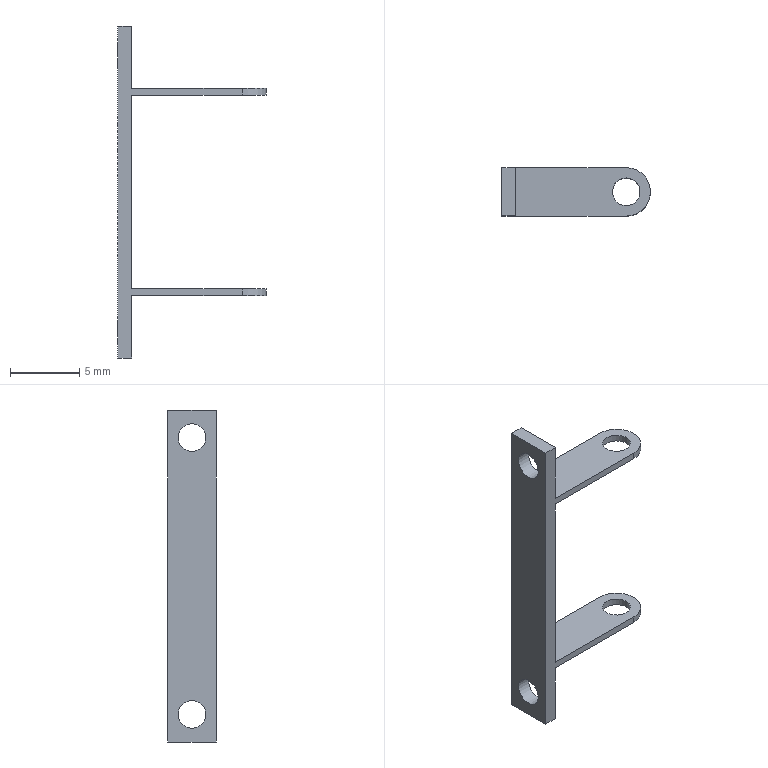Part | STEP file | 1-63.3 | 1 solid | 18 faces | box 10.75 x 3.5 x 24 mm | volume 107.386 mm3 | plane 12 | cylinder 6 | commonest cylinder face diameters 2 x4 3.5 x2
STEP:
#1=CARTESIAN_POINT('',(0.,0.,0.));
#2=DIRECTION('',(0.,0.,1.));
#3=DIRECTION('',(1.,0.,0.));
#4=AXIS2_PLACEMENT_3D('',#1,#2,#3);
#5=CARTESIAN_POINT('',(0.,-1.75,-12.));
#6=VERTEX_POINT('',#5);
#7=CARTESIAN_POINT('',(0.,1.75,-12.));
#8=VERTEX_POINT('',#7);
#9=CARTESIAN_POINT('',(0.,-1.75,-12.));
#10=DIRECTION('',(0.,1.,0.));
#11=VECTOR('',#10,1.);
#12=LINE('',#9,#11);
#13=CARTESIAN_POINT('',(0.,10.25,0.));
#14=DIRECTION('',(1.,0.,0.));
#15=DIRECTION('',(0.,1.,0.));
#16=AXIS2_PLACEMENT_3D('',#13,#14,#15);
#17=PLANE('',#16);
#18=CARTESIAN_POINT('',(-12.,-12.));
#19=DIRECTION('',(1.,0.));
#20=VECTOR('',#19,1.);
#21=LINE('',#18,#20);
#22=(GEOMETRIC_REPRESENTATION_CONTEXT(2)PARAMETRIC_REPRESENTATION_CONTEXT()REPRESENTATION_CONTEXT('',''));
#23=DEFINITIONAL_REPRESENTATION('',(#21),#22);
#24=PCURVE('',#17,#23);
#25=CARTESIAN_POINT('',(0.5,0.,-12.));
#26=DIRECTION('',(0.,0.,-1.));
#27=DIRECTION('',(0.,1.,0.));
#28=AXIS2_PLACEMENT_3D('',#25,#26,#27);
#29=PLANE('',#28);
#30=CARTESIAN_POINT('',(-1.75,-0.5));
#31=DIRECTION('',(1.,0.));
#32=VECTOR('',#31,1.);
#33=LINE('',#30,#32);
#34=(GEOMETRIC_REPRESENTATION_CONTEXT(2)PARAMETRIC_REPRESENTATION_CONTEXT()REPRESENTATION_CONTEXT('',''));
#35=DEFINITIONAL_REPRESENTATION('',(#33),#34);
#36=PCURVE('',#29,#35);
#37=SURFACE_CURVE('',#12,(#24,#36),.PCURVE_S1.);
#38=EDGE_CURVE('',#6,#8,#37,.T.);
#39=ORIENTED_EDGE('',*,*,#38,.T.);
#40=CARTESIAN_POINT('',(0.,1.75,12.));
#41=VERTEX_POINT('',#40);
#42=CARTESIAN_POINT('',(0.,1.75,-12.));
#43=DIRECTION('',(0.,0.,1.));
#44=VECTOR('',#43,1.);
#45=LINE('',#42,#44);
#46=CARTESIAN_POINT('',(-8.5,-12.));
#47=DIRECTION('',(0.,1.));
#48=VECTOR('',#47,1.);
#49=LINE('',#46,#48);
#50=(GEOMETRIC_REPRESENTATION_CONTEXT(2)PARAMETRIC_REPRESENTATION_CONTEXT()REPRESENTATION_CONTEXT('',''));
#51=DEFINITIONAL_REPRESENTATION('',(#49),#50);
#52=PCURVE('',#17,#51);
#53=CARTESIAN_POINT('',(4.5,1.75,0.));
#54=DIRECTION('',(0.,1.,0.));
#55=DIRECTION('',(0.,0.,1.));
#56=AXIS2_PLACEMENT_3D('',#53,#54,#55);
#57=PLANE('',#56);
#58=CARTESIAN_POINT('',(-12.,-4.5));
#59=DIRECTION('',(1.,0.));
#60=VECTOR('',#59,1.);
#61=LINE('',#58,#60);
#62=(GEOMETRIC_REPRESENTATION_CONTEXT(2)PARAMETRIC_REPRESENTATION_CONTEXT()REPRESENTATION_CONTEXT('',''));
#63=DEFINITIONAL_REPRESENTATION('',(#61),#62);
#64=PCURVE('',#57,#63);
#65=SURFACE_CURVE('',#45,(#52,#64),.PCURVE_S1.);
#66=EDGE_CURVE('',#8,#41,#65,.T.);
#67=ORIENTED_EDGE('',*,*,#66,.T.);
#68=CARTESIAN_POINT('',(0.,-1.75,12.));
#69=VERTEX_POINT('',#68);
#70=CARTESIAN_POINT('',(0.,1.75,12.));
#71=DIRECTION('',(0.,-1.,0.));
#72=VECTOR('',#71,1.);
#73=LINE('',#70,#72);
#74=CARTESIAN_POINT('',(-8.5,12.));
#75=DIRECTION('',(-1.,0.));
#76=VECTOR('',#75,1.);
#77=LINE('',#74,#76);
#78=(GEOMETRIC_REPRESENTATION_CONTEXT(2)PARAMETRIC_REPRESENTATION_CONTEXT()REPRESENTATION_CONTEXT('',''));
#79=DEFINITIONAL_REPRESENTATION('',(#77),#78);
#80=PCURVE('',#17,#79);
#81=CARTESIAN_POINT('',(0.5,0.,12.));
#82=DIRECTION('',(0.,0.,1.));
#83=DIRECTION('',(0.,-1.,0.));
#84=AXIS2_PLACEMENT_3D('',#81,#82,#83);
#85=PLANE('',#84);
#86=CARTESIAN_POINT('',(-1.75,-0.5));
#87=DIRECTION('',(1.,0.));
#88=VECTOR('',#87,1.);
#89=LINE('',#86,#88);
#90=(GEOMETRIC_REPRESENTATION_CONTEXT(2)PARAMETRIC_REPRESENTATION_CONTEXT()REPRESENTATION_CONTEXT('',''));
#91=DEFINITIONAL_REPRESENTATION('',(#89),#90);
#92=PCURVE('',#85,#91);
#93=SURFACE_CURVE('',#73,(#80,#92),.PCURVE_S1.);
#94=EDGE_CURVE('',#41,#69,#93,.T.);
#95=ORIENTED_EDGE('',*,*,#94,.T.);
#96=CARTESIAN_POINT('',(0.,-1.75,12.));
#97=DIRECTION('',(0.,0.,-1.));
#98=VECTOR('',#97,1.);
#99=LINE('',#96,#98);
#100=CARTESIAN_POINT('',(-12.,12.));
#101=DIRECTION('',(0.,-1.));
#102=VECTOR('',#101,1.);
#103=LINE('',#100,#102);
#104=(GEOMETRIC_REPRESENTATION_CONTEXT(2)PARAMETRIC_REPRESENTATION_CONTEXT()REPRESENTATION_CONTEXT('',''));
#105=DEFINITIONAL_REPRESENTATION('',(#103),#104);
#106=PCURVE('',#17,#105);
#107=CARTESIAN_POINT('',(4.5,-1.75,0.));
#108=DIRECTION('',(0.,-1.,0.));
#109=DIRECTION('',(0.,0.,-1.));
#110=AXIS2_PLACEMENT_3D('',#107,#108,#109);
#111=PLANE('',#110);
#112=CARTESIAN_POINT('',(-12.,-4.5));
#113=DIRECTION('',(1.,0.));
#114=VECTOR('',#113,1.);
#115=LINE('',#112,#114);
#116=(GEOMETRIC_REPRESENTATION_CONTEXT(2)PARAMETRIC_REPRESENTATION_CONTEXT()REPRESENTATION_CONTEXT('',''));
#117=DEFINITIONAL_REPRESENTATION('',(#115),#116);
#118=PCURVE('',#111,#117);
#119=SURFACE_CURVE('',#99,(#106,#118),.PCURVE_S1.);
#120=EDGE_CURVE('',#69,#6,#119,.T.);
#121=ORIENTED_EDGE('',*,*,#120,.T.);
#122=EDGE_LOOP('',(#39,#67,#95,#121));
#123=FACE_BOUND('',#122,.F.);
#124=CARTESIAN_POINT('',(0.,1.,10.));
#125=VERTEX_POINT('',#124);
#126=CARTESIAN_POINT('',(0.,0.,10.));
#127=DIRECTION('',(-1.,0.,0.));
#128=DIRECTION('',(0.,1.,0.));
#129=AXIS2_PLACEMENT_3D('',#126,#127,#128);
#130=CIRCLE('',#129,1.);
#131=CARTESIAN_POINT('',(-9.25,10.));
#132=CARTESIAN_POINT('',(-9.25,8.268));
#133=CARTESIAN_POINT('',(-10.75,9.134));
#134=CARTESIAN_POINT('',(-12.25,10.));
#135=CARTESIAN_POINT('',(-10.75,10.866));
#136=CARTESIAN_POINT('',(-9.25,11.732));
#137=CARTESIAN_POINT('',(-9.25,10.));
#138=(BOUNDED_CURVE()B_SPLINE_CURVE(2,(#131,#132,#133,#134,#135,#136,#137),.UNSPECIFIED.,.T.,.F.)B_SPLINE_CURVE_WITH_KNOTS((1,2,2,2,2,1),(-2.094,0.,2.094,4.189,6.283,8.378),.UNSPECIFIED.)CURVE()GEOMETRIC_REPRESENTATION_ITEM()RATIONAL_B_SPLINE_CURVE((1.,0.5,1.,0.5,1.,0.5,1.))REPRESENTATION_ITEM(''));
#139=(GEOMETRIC_REPRESENTATION_CONTEXT(2)PARAMETRIC_REPRESENTATION_CONTEXT()REPRESENTATION_CONTEXT('',''));
#140=DEFINITIONAL_REPRESENTATION('',(#138),#139);
#141=PCURVE('',#17,#140);
#142=CARTESIAN_POINT('',(0.,0.,10.));
#143=DIRECTION('',(1.,0.,0.));
#144=DIRECTION('',(0.,1.,0.));
#145=AXIS2_PLACEMENT_3D('',#142,#143,#144);
#146=CYLINDRICAL_SURFACE('',#145,1.);
#147=CARTESIAN_POINT('',(6.283,0.));
#148=DIRECTION('',(-1.,0.));
#149=VECTOR('',#148,1.);
#150=LINE('',#147,#149);
#151=(GEOMETRIC_REPRESENTATION_CONTEXT(2)PARAMETRIC_REPRESENTATION_CONTEXT()REPRESENTATION_CONTEXT('',''));
#152=DEFINITIONAL_REPRESENTATION('',(#150),#151);
#153=PCURVE('',#146,#152);
#154=SURFACE_CURVE('',#130,(#141,#153),.PCURVE_S1.);
#155=EDGE_CURVE('',#125,#125,#154,.T.);
#156=ORIENTED_EDGE('',*,*,#155,.T.);
#157=EDGE_LOOP('',(#156));
#158=FACE_BOUND('',#157,.F.);
#159=CARTESIAN_POINT('',(0.,1.,-10.));
#160=VERTEX_POINT('',#159);
#161=CARTESIAN_POINT('',(0.,0.,-10.));
#162=DIRECTION('',(-1.,0.,0.));
#163=DIRECTION('',(0.,1.,0.));
#164=AXIS2_PLACEMENT_3D('',#161,#162,#163);
#165=CIRCLE('',#164,1.);
#166=CARTESIAN_POINT('',(-9.25,-10.));
#167=CARTESIAN_POINT('',(-9.25,-11.732));
#168=CARTESIAN_POINT('',(-10.75,-10.866));
#169=CARTESIAN_POINT('',(-12.25,-10.));
#170=CARTESIAN_POINT('',(-10.75,-9.134));
#171=CARTESIAN_POINT('',(-9.25,-8.268));
#172=CARTESIAN_POINT('',(-9.25,-10.));
#173=(BOUNDED_CURVE()B_SPLINE_CURVE(2,(#166,#167,#168,#169,#170,#171,#172),.UNSPECIFIED.,.T.,.F.)B_SPLINE_CURVE_WITH_KNOTS((1,2,2,2,2,1),(-2.094,0.,2.094,4.189,6.283,8.378),.UNSPECIFIED.)CURVE()GEOMETRIC_REPRESENTATION_ITEM()RATIONAL_B_SPLINE_CURVE((1.,0.5,1.,0.5,1.,0.5,1.))REPRESENTATION_ITEM(''));
#174=(GEOMETRIC_REPRESENTATION_CONTEXT(2)PARAMETRIC_REPRESENTATION_CONTEXT()REPRESENTATION_CONTEXT('',''));
#175=DEFINITIONAL_REPRESENTATION('',(#173),#174);
#176=PCURVE('',#17,#175);
#177=CARTESIAN_POINT('',(0.,0.,-10.));
#178=DIRECTION('',(1.,0.,0.));
#179=DIRECTION('',(0.,1.,0.));
#180=AXIS2_PLACEMENT_3D('',#177,#178,#179);
#181=CYLINDRICAL_SURFACE('',#180,1.);
#182=CARTESIAN_POINT('',(6.283,0.));
#183=DIRECTION('',(-1.,0.));
#184=VECTOR('',#183,1.);
#185=LINE('',#182,#184);
#186=(GEOMETRIC_REPRESENTATION_CONTEXT(2)PARAMETRIC_REPRESENTATION_CONTEXT()REPRESENTATION_CONTEXT('',''));
#187=DEFINITIONAL_REPRESENTATION('',(#185),#186);
#188=PCURVE('',#181,#187);
#189=SURFACE_CURVE('',#165,(#176,#188),.PCURVE_S1.);
#190=EDGE_CURVE('',#160,#160,#189,.T.);
#191=ORIENTED_EDGE('',*,*,#190,.T.);
#192=EDGE_LOOP('',(#191));
#193=FACE_BOUND('',#192,.F.);
#194=ADVANCED_FACE('',(#123,#158,#193),#17,.F.);
#195=ORIENTED_EDGE('',*,*,#38,.T.);
#196=CARTESIAN_POINT('',(1.,1.75,-12.));
#197=VERTEX_POINT('',#196);
#198=CARTESIAN_POINT('',(0.,1.75,-12.));
#199=DIRECTION('',(1.,0.,0.));
#200=VECTOR('',#199,1.);
#201=LINE('',#198,#200);
#202=CARTESIAN_POINT('',(1.75,-0.5));
#203=DIRECTION('',(0.,1.));
#204=VECTOR('',#203,1.);
#205=LINE('',#202,#204);
#206=(GEOMETRIC_REPRESENTATION_CONTEXT(2)PARAMETRIC_REPRESENTATION_CONTEXT()REPRESENTATION_CONTEXT('',''));
#207=DEFINITIONAL_REPRESENTATION('',(#205),#206);
#208=PCURVE('',#29,#207);
#209=CARTESIAN_POINT('',(-12.,-4.5));
#210=DIRECTION('',(0.,1.));
#211=VECTOR('',#210,1.);
#212=LINE('',#209,#211);
#213=(GEOMETRIC_REPRESENTATION_CONTEXT(2)PARAMETRIC_REPRESENTATION_CONTEXT()REPRESENTATION_CONTEXT('',''));
#214=DEFINITIONAL_REPRESENTATION('',(#212),#213);
#215=PCURVE('',#57,#214);
#216=SURFACE_CURVE('',#201,(#208,#215),.PCURVE_S1.);
#217=EDGE_CURVE('',#8,#197,#216,.T.);
#218=ORIENTED_EDGE('',*,*,#217,.T.);
#219=CARTESIAN_POINT('',(1.,-1.75,-12.));
#220=VERTEX_POINT('',#219);
#221=CARTESIAN_POINT('',(1.,-1.75,-12.));
#222=DIRECTION('',(0.,1.,0.));
#223=VECTOR('',#222,1.);
#224=LINE('',#221,#223);
#225=CARTESIAN_POINT('',(-1.75,0.5));
#226=DIRECTION('',(1.,0.));
#227=VECTOR('',#226,1.);
#228=LINE('',#225,#227);
#229=(GEOMETRIC_REPRESENTATION_CONTEXT(2)PARAMETRIC_REPRESENTATION_CONTEXT()REPRESENTATION_CONTEXT('',''));
#230=DEFINITIONAL_REPRESENTATION('',(#228),#229);
#231=PCURVE('',#29,#230);
#232=CARTESIAN_POINT('',(1.,0.,0.));
#233=DIRECTION('',(1.,0.,0.));
#234=DIRECTION('',(0.,1.,0.));
#235=AXIS2_PLACEMENT_3D('',#232,#233,#234);
#236=PLANE('',#235);
#237=CARTESIAN_POINT('',(-1.75,-12.));
#238=DIRECTION('',(1.,0.));
#239=VECTOR('',#238,1.);
#240=LINE('',#237,#239);
#241=(GEOMETRIC_REPRESENTATION_CONTEXT(2)PARAMETRIC_REPRESENTATION_CONTEXT()REPRESENTATION_CONTEXT('',''));
#242=DEFINITIONAL_REPRESENTATION('',(#240),#241);
#243=PCURVE('',#236,#242);
#244=SURFACE_CURVE('',#224,(#231,#243),.PCURVE_S1.);
#245=EDGE_CURVE('',#220,#197,#244,.T.);
#246=ORIENTED_EDGE('',*,*,#245,.F.);
#247=CARTESIAN_POINT('',(0.,-1.75,-12.));
#248=DIRECTION('',(1.,0.,0.));
#249=VECTOR('',#248,1.);
#250=LINE('',#247,#249);
#251=CARTESIAN_POINT('',(-1.75,-0.5));
#252=DIRECTION('',(0.,1.));
#253=VECTOR('',#252,1.);
#254=LINE('',#251,#253);
#255=(GEOMETRIC_REPRESENTATION_CONTEXT(2)PARAMETRIC_REPRESENTATION_CONTEXT()REPRESENTATION_CONTEXT('',''));
#256=DEFINITIONAL_REPRESENTATION('',(#254),#255);
#257=PCURVE('',#29,#256);
#258=CARTESIAN_POINT('',(12.,-4.5));
#259=DIRECTION('',(0.,1.));
#260=VECTOR('',#259,1.);
#261=LINE('',#258,#260);
#262=(GEOMETRIC_REPRESENTATION_CONTEXT(2)PARAMETRIC_REPRESENTATION_CONTEXT()REPRESENTATION_CONTEXT('',''));
#263=DEFINITIONAL_REPRESENTATION('',(#261),#262);
#264=PCURVE('',#111,#263);
#265=SURFACE_CURVE('',#250,(#257,#264),.PCURVE_S1.);
#266=EDGE_CURVE('',#6,#220,#265,.T.);
#267=ORIENTED_EDGE('',*,*,#266,.F.);
#268=EDGE_LOOP('',(#195,#218,#246,#267));
#269=FACE_BOUND('',#268,.T.);
#270=ADVANCED_FACE('',(#269),#29,.T.);
#271=ORIENTED_EDGE('',*,*,#94,.T.);
#272=CARTESIAN_POINT('',(1.,-1.75,12.));
#273=VERTEX_POINT('',#272);
#274=CARTESIAN_POINT('',(0.,-1.75,12.));
#275=DIRECTION('',(1.,0.,0.));
#276=VECTOR('',#275,1.);
#277=LINE('',#274,#276);
#278=CARTESIAN_POINT('',(1.75,-0.5));
#279=DIRECTION('',(0.,1.));
#280=VECTOR('',#279,1.);
#281=LINE('',#278,#280);
#282=(GEOMETRIC_REPRESENTATION_CONTEXT(2)PARAMETRIC_REPRESENTATION_CONTEXT()REPRESENTATION_CONTEXT('',''));
#283=DEFINITIONAL_REPRESENTATION('',(#281),#282);
#284=PCURVE('',#85,#283);
#285=CARTESIAN_POINT('',(-12.,-4.5));
#286=DIRECTION('',(0.,1.));
#287=VECTOR('',#286,1.);
#288=LINE('',#285,#287);
#289=(GEOMETRIC_REPRESENTATION_CONTEXT(2)PARAMETRIC_REPRESENTATION_CONTEXT()REPRESENTATION_CONTEXT('',''));
#290=DEFINITIONAL_REPRESENTATION('',(#288),#289);
#291=PCURVE('',#111,#290);
#292=SURFACE_CURVE('',#277,(#284,#291),.PCURVE_S1.);
#293=EDGE_CURVE('',#69,#273,#292,.T.);
#294=ORIENTED_EDGE('',*,*,#293,.T.);
#295=CARTESIAN_POINT('',(1.,1.75,12.));
#296=VERTEX_POINT('',#295);
#297=CARTESIAN_POINT('',(1.,1.75,12.));
#298=DIRECTION('',(0.,-1.,0.));
#299=VECTOR('',#298,1.);
#300=LINE('',#297,#299);
#301=CARTESIAN_POINT('',(-1.75,0.5));
#302=DIRECTION('',(1.,0.));
#303=VECTOR('',#302,1.);
#304=LINE('',#301,#303);
#305=(GEOMETRIC_REPRESENTATION_CONTEXT(2)PARAMETRIC_REPRESENTATION_CONTEXT()REPRESENTATION_CONTEXT('',''));
#306=DEFINITIONAL_REPRESENTATION('',(#304),#305);
#307=PCURVE('',#85,#306);
#308=CARTESIAN_POINT('',(1.,0.,0.));
#309=DIRECTION('',(1.,0.,0.));
#310=DIRECTION('',(0.,1.,0.));
#311=AXIS2_PLACEMENT_3D('',#308,#309,#310);
#312=PLANE('',#311);
#313=CARTESIAN_POINT('',(1.75,12.));
#314=DIRECTION('',(-1.,0.));
#315=VECTOR('',#314,1.);
#316=LINE('',#313,#315);
#317=(GEOMETRIC_REPRESENTATION_CONTEXT(2)PARAMETRIC_REPRESENTATION_CONTEXT()REPRESENTATION_CONTEXT('',''));
#318=DEFINITIONAL_REPRESENTATION('',(#316),#317);
#319=PCURVE('',#312,#318);
#320=SURFACE_CURVE('',#300,(#307,#319),.PCURVE_S1.);
#321=EDGE_CURVE('',#296,#273,#320,.T.);
#322=ORIENTED_EDGE('',*,*,#321,.F.);
#323=CARTESIAN_POINT('',(0.,1.75,12.));
#324=DIRECTION('',(1.,0.,0.));
#325=VECTOR('',#324,1.);
#326=LINE('',#323,#325);
#327=CARTESIAN_POINT('',(-1.75,-0.5));
#328=DIRECTION('',(0.,1.));
#329=VECTOR('',#328,1.);
#330=LINE('',#327,#329);
#331=(GEOMETRIC_REPRESENTATION_CONTEXT(2)PARAMETRIC_REPRESENTATION_CONTEXT()REPRESENTATION_CONTEXT('',''));
#332=DEFINITIONAL_REPRESENTATION('',(#330),#331);
#333=PCURVE('',#85,#332);
#334=CARTESIAN_POINT('',(12.,-4.5));
#335=DIRECTION('',(0.,1.));
#336=VECTOR('',#335,1.);
#337=LINE('',#334,#336);
#338=(GEOMETRIC_REPRESENTATION_CONTEXT(2)PARAMETRIC_REPRESENTATION_CONTEXT()REPRESENTATION_CONTEXT('',''));
#339=DEFINITIONAL_REPRESENTATION('',(#337),#338);
#340=PCURVE('',#57,#339);
#341=SURFACE_CURVE('',#326,(#333,#340),.PCURVE_S1.);
#342=EDGE_CURVE('',#41,#296,#341,.T.);
#343=ORIENTED_EDGE('',*,*,#342,.F.);
#344=EDGE_LOOP('',(#271,#294,#322,#343));
#345=FACE_BOUND('',#344,.T.);
#346=ADVANCED_FACE('',(#345),#85,.T.);
#347=CARTESIAN_POINT('',(1.,1.,10.));
#348=VERTEX_POINT('',#347);
#349=CARTESIAN_POINT('',(0.,1.,10.));
#350=DIRECTION('',(1.,0.,0.));
#351=VECTOR('',#350,1.);
#352=LINE('',#349,#351);
#353=CARTESIAN_POINT('',(6.283,0.));
#354=DIRECTION('',(0.,1.));
#355=VECTOR('',#354,1.);
#356=LINE('',#353,#355);
#357=(GEOMETRIC_REPRESENTATION_CONTEXT(2)PARAMETRIC_REPRESENTATION_CONTEXT()REPRESENTATION_CONTEXT('',''));
#358=DEFINITIONAL_REPRESENTATION('',(#356),#357);
#359=PCURVE('',#146,#358);
#360=CARTESIAN_POINT('',(0.,0.));
#361=DIRECTION('',(0.,1.));
#362=VECTOR('',#361,1.);
#363=LINE('',#360,#362);
#364=(GEOMETRIC_REPRESENTATION_CONTEXT(2)PARAMETRIC_REPRESENTATION_CONTEXT()REPRESENTATION_CONTEXT('',''));
#365=DEFINITIONAL_REPRESENTATION('',(#363),#364);
#366=PCURVE('',#146,#365);
#367=SEAM_CURVE('',#352,(#359,#366),.PCURVE_S1.);
#368=EDGE_CURVE('',#125,#348,#367,.T.);
#369=ORIENTED_EDGE('',*,*,#368,.T.);
#370=CARTESIAN_POINT('',(1.,0.,10.));
#371=DIRECTION('',(-1.,0.,0.));
#372=DIRECTION('',(0.,1.,0.));
#373=AXIS2_PLACEMENT_3D('',#370,#371,#372);
#374=CIRCLE('',#373,1.);
#375=CARTESIAN_POINT('',(6.283,1.));
#376=DIRECTION('',(-1.,0.));
#377=VECTOR('',#376,1.);
#378=LINE('',#375,#377);
#379=(GEOMETRIC_REPRESENTATION_CONTEXT(2)PARAMETRIC_REPRESENTATION_CONTEXT()REPRESENTATION_CONTEXT('',''));
#380=DEFINITIONAL_REPRESENTATION('',(#378),#379);
#381=PCURVE('',#146,#380);
#382=CARTESIAN_POINT('',(1.,10.));
#383=CARTESIAN_POINT('',(1.,8.268));
#384=CARTESIAN_POINT('',(-0.5,9.134));
#385=CARTESIAN_POINT('',(-2.,10.));
#386=CARTESIAN_POINT('',(-0.5,10.866));
#387=CARTESIAN_POINT('',(1.,11.732));
#388=CARTESIAN_POINT('',(1.,10.));
#389=(BOUNDED_CURVE()B_SPLINE_CURVE(2,(#382,#383,#384,#385,#386,#387,#388),.UNSPECIFIED.,.T.,.F.)B_SPLINE_CURVE_WITH_KNOTS((1,2,2,2,2,1),(-2.094,0.,2.094,4.189,6.283,8.378),.UNSPECIFIED.)CURVE()GEOMETRIC_REPRESENTATION_ITEM()RATIONAL_B_SPLINE_CURVE((1.,0.5,1.,0.5,1.,0.5,1.))REPRESENTATION_ITEM(''));
#390=(GEOMETRIC_REPRESENTATION_CONTEXT(2)PARAMETRIC_REPRESENTATION_CONTEXT()REPRESENTATION_CONTEXT('',''));
#391=DEFINITIONAL_REPRESENTATION('',(#389),#390);
#392=PCURVE('',#312,#391);
#393=SURFACE_CURVE('',#374,(#381,#392),.PCURVE_S1.);
#394=EDGE_CURVE('',#348,#348,#393,.T.);
#395=ORIENTED_EDGE('',*,*,#394,.T.);
#396=ORIENTED_EDGE('',*,*,#368,.F.);
#397=ORIENTED_EDGE('',*,*,#155,.F.);
#398=EDGE_LOOP('',(#369,#395,#396,#397));
#399=FACE_BOUND('',#398,.F.);
#400=ADVANCED_FACE('',(#399),#146,.F.);
#401=CARTESIAN_POINT('',(1.,1.,-10.));
#402=VERTEX_POINT('',#401);
#403=CARTESIAN_POINT('',(0.,1.,-10.));
#404=DIRECTION('',(1.,0.,0.));
#405=VECTOR('',#404,1.);
#406=LINE('',#403,#405);
#407=CARTESIAN_POINT('',(6.283,0.));
#408=DIRECTION('',(0.,1.));
#409=VECTOR('',#408,1.);
#410=LINE('',#407,#409);
#411=(GEOMETRIC_REPRESENTATION_CONTEXT(2)PARAMETRIC_REPRESENTATION_CONTEXT()REPRESENTATION_CONTEXT('',''));
#412=DEFINITIONAL_REPRESENTATION('',(#410),#411);
#413=PCURVE('',#181,#412);
#414=CARTESIAN_POINT('',(0.,0.));
#415=DIRECTION('',(0.,1.));
#416=VECTOR('',#415,1.);
#417=LINE('',#414,#416);
#418=(GEOMETRIC_REPRESENTATION_CONTEXT(2)PARAMETRIC_REPRESENTATION_CONTEXT()REPRESENTATION_CONTEXT('',''));
#419=DEFINITIONAL_REPRESENTATION('',(#417),#418);
#420=PCURVE('',#181,#419);
#421=SEAM_CURVE('',#406,(#413,#420),.PCURVE_S1.);
#422=EDGE_CURVE('',#160,#402,#421,.T.);
#423=ORIENTED_EDGE('',*,*,#422,.T.);
#424=CARTESIAN_POINT('',(1.,0.,-10.));
#425=DIRECTION('',(-1.,0.,0.));
#426=DIRECTION('',(0.,1.,0.));
#427=AXIS2_PLACEMENT_3D('',#424,#425,#426);
#428=CIRCLE('',#427,1.);
#429=CARTESIAN_POINT('',(6.283,1.));
#430=DIRECTION('',(-1.,0.));
#431=VECTOR('',#430,1.);
#432=LINE('',#429,#431);
#433=(GEOMETRIC_REPRESENTATION_CONTEXT(2)PARAMETRIC_REPRESENTATION_CONTEXT()REPRESENTATION_CONTEXT('',''));
#434=DEFINITIONAL_REPRESENTATION('',(#432),#433);
#435=PCURVE('',#181,#434);
#436=CARTESIAN_POINT('',(1.,-10.));
#437=CARTESIAN_POINT('',(1.,-11.732));
#438=CARTESIAN_POINT('',(-0.5,-10.866));
#439=CARTESIAN_POINT('',(-2.,-10.));
#440=CARTESIAN_POINT('',(-0.5,-9.134));
#441=CARTESIAN_POINT('',(1.,-8.268));
#442=CARTESIAN_POINT('',(1.,-10.));
#443=(BOUNDED_CURVE()B_SPLINE_CURVE(2,(#436,#437,#438,#439,#440,#441,#442),.UNSPECIFIED.,.T.,.F.)B_SPLINE_CURVE_WITH_KNOTS((1,2,2,2,2,1),(-2.094,0.,2.094,4.189,6.283,8.378),.UNSPECIFIED.)CURVE()GEOMETRIC_REPRESENTATION_ITEM()RATIONAL_B_SPLINE_CURVE((1.,0.5,1.,0.5,1.,0.5,1.))REPRESENTATION_ITEM(''));
#444=(GEOMETRIC_REPRESENTATION_CONTEXT(2)PARAMETRIC_REPRESENTATION_CONTEXT()REPRESENTATION_CONTEXT('',''));
#445=DEFINITIONAL_REPRESENTATION('',(#443),#444);
#446=PCURVE('',#236,#445);
#447=SURFACE_CURVE('',#428,(#435,#446),.PCURVE_S1.);
#448=EDGE_CURVE('',#402,#402,#447,.T.);
#449=ORIENTED_EDGE('',*,*,#448,.T.);
#450=ORIENTED_EDGE('',*,*,#422,.F.);
#451=ORIENTED_EDGE('',*,*,#190,.F.);
#452=EDGE_LOOP('',(#423,#449,#450,#451));
#453=FACE_BOUND('',#452,.F.);
#454=ADVANCED_FACE('',(#453),#181,.F.);
#455=ORIENTED_EDGE('',*,*,#245,.T.);
#456=CARTESIAN_POINT('',(1.,1.75,-7.5));
#457=VERTEX_POINT('',#456);
#458=CARTESIAN_POINT('',(1.,1.75,-12.));
#459=DIRECTION('',(0.,0.,1.));
#460=VECTOR('',#459,1.);
#461=LINE('',#458,#460);
#462=CARTESIAN_POINT('',(1.75,-12.));
#463=DIRECTION('',(0.,1.));
#464=VECTOR('',#463,1.);
#465=LINE('',#462,#464);
#466=(GEOMETRIC_REPRESENTATION_CONTEXT(2)PARAMETRIC_REPRESENTATION_CONTEXT()REPRESENTATION_CONTEXT('',''));
#467=DEFINITIONAL_REPRESENTATION('',(#465),#466);
#468=PCURVE('',#236,#467);
#469=CARTESIAN_POINT('',(-12.,-3.5));
#470=DIRECTION('',(1.,0.));
#471=VECTOR('',#470,1.);
#472=LINE('',#469,#471);
#473=(GEOMETRIC_REPRESENTATION_CONTEXT(2)PARAMETRIC_REPRESENTATION_CONTEXT()REPRESENTATION_CONTEXT('',''));
#474=DEFINITIONAL_REPRESENTATION('',(#472),#473);
#475=PCURVE('',#57,#474);
#476=SURFACE_CURVE('',#461,(#468,#475),.PCURVE_S1.);
#477=EDGE_CURVE('',#197,#457,#476,.T.);
#478=ORIENTED_EDGE('',*,*,#477,.T.);
#479=CARTESIAN_POINT('',(1.,-1.75,-7.5));
#480=VERTEX_POINT('',#479);
#481=CARTESIAN_POINT('',(1.,1.75,-7.5));
#482=DIRECTION('',(0.,-1.,0.));
#483=VECTOR('',#482,1.);
#484=LINE('',#481,#483);
#485=CARTESIAN_POINT('',(1.75,-7.5));
#486=DIRECTION('',(-1.,0.));
#487=VECTOR('',#486,1.);
#488=LINE('',#485,#487);
#489=(GEOMETRIC_REPRESENTATION_CONTEXT(2)PARAMETRIC_REPRESENTATION_CONTEXT()REPRESENTATION_CONTEXT('',''));
#490=DEFINITIONAL_REPRESENTATION('',(#488),#489);
#491=PCURVE('',#236,#490);
#492=CARTESIAN_POINT('',(5.875,3.125,-7.5));
#493=DIRECTION('',(0.,0.,1.));
#494=DIRECTION('',(0.,1.,0.));
#495=AXIS2_PLACEMENT_3D('',#492,#493,#494);
#496=PLANE('',#495);
#497=CARTESIAN_POINT('',(-1.375,4.875));
#498=DIRECTION('',(-1.,0.));
#499=VECTOR('',#498,1.);
#500=LINE('',#497,#499);
#501=(GEOMETRIC_REPRESENTATION_CONTEXT(2)PARAMETRIC_REPRESENTATION_CONTEXT()REPRESENTATION_CONTEXT('',''));
#502=DEFINITIONAL_REPRESENTATION('',(#500),#501);
#503=PCURVE('',#496,#502);
#504=SURFACE_CURVE('',#484,(#491,#503),.PCURVE_S1.);
#505=EDGE_CURVE('',#457,#480,#504,.T.);
#506=ORIENTED_EDGE('',*,*,#505,.T.);
#507=CARTESIAN_POINT('',(1.,-1.75,-7.5));
#508=DIRECTION('',(0.,0.,-1.));
#509=VECTOR('',#508,1.);
#510=LINE('',#507,#509);
#511=CARTESIAN_POINT('',(-1.75,-7.5));
#512=DIRECTION('',(0.,-1.));
#513=VECTOR('',#512,1.);
#514=LINE('',#511,#513);
#515=(GEOMETRIC_REPRESENTATION_CONTEXT(2)PARAMETRIC_REPRESENTATION_CONTEXT()REPRESENTATION_CONTEXT('',''));
#516=DEFINITIONAL_REPRESENTATION('',(#514),#515);
#517=PCURVE('',#236,#516);
#518=CARTESIAN_POINT('',(7.5,-3.5));
#519=DIRECTION('',(1.,0.));
#520=VECTOR('',#519,1.);
#521=LINE('',#518,#520);
#522=(GEOMETRIC_REPRESENTATION_CONTEXT(2)PARAMETRIC_REPRESENTATION_CONTEXT()REPRESENTATION_CONTEXT('',''));
#523=DEFINITIONAL_REPRESENTATION('',(#521),#522);
#524=PCURVE('',#111,#523);
#525=SURFACE_CURVE('',#510,(#517,#524),.PCURVE_S1.);
#526=EDGE_CURVE('',#480,#220,#525,.T.);
#527=ORIENTED_EDGE('',*,*,#526,.T.);
#528=EDGE_LOOP('',(#455,#478,#506,#527));
#529=FACE_BOUND('',#528,.T.);
#530=ORIENTED_EDGE('',*,*,#448,.T.);
#531=EDGE_LOOP('',(#530));
#532=FACE_BOUND('',#531,.T.);
#533=ADVANCED_FACE('',(#529,#532),#236,.T.);
#534=ORIENTED_EDGE('',*,*,#321,.T.);
#535=CARTESIAN_POINT('',(1.,-1.75,7.5));
#536=VERTEX_POINT('',#535);
#537=CARTESIAN_POINT('',(1.,-1.75,12.));
#538=DIRECTION('',(0.,0.,-1.));
#539=VECTOR('',#538,1.);
#540=LINE('',#537,#539);
#541=CARTESIAN_POINT('',(-1.75,12.));
#542=DIRECTION('',(0.,-1.));
#543=VECTOR('',#542,1.);
#544=LINE('',#541,#543);
#545=(GEOMETRIC_REPRESENTATION_CONTEXT(2)PARAMETRIC_REPRESENTATION_CONTEXT()REPRESENTATION_CONTEXT('',''));
#546=DEFINITIONAL_REPRESENTATION('',(#544),#545);
#547=PCURVE('',#312,#546);
#548=CARTESIAN_POINT('',(-12.,-3.5));
#549=DIRECTION('',(1.,0.));
#550=VECTOR('',#549,1.);
#551=LINE('',#548,#550);
#552=(GEOMETRIC_REPRESENTATION_CONTEXT(2)PARAMETRIC_REPRESENTATION_CONTEXT()REPRESENTATION_CONTEXT('',''));
#553=DEFINITIONAL_REPRESENTATION('',(#551),#552);
#554=PCURVE('',#111,#553);
#555=SURFACE_CURVE('',#540,(#547,#554),.PCURVE_S1.);
#556=EDGE_CURVE('',#273,#536,#555,.T.);
#557=ORIENTED_EDGE('',*,*,#556,.T.);
#558=CARTESIAN_POINT('',(1.,1.75,7.5));
#559=VERTEX_POINT('',#558);
#560=CARTESIAN_POINT('',(1.,1.75,7.5));
#561=DIRECTION('',(0.,-1.,0.));
#562=VECTOR('',#561,1.);
#563=LINE('',#560,#562);
#564=CARTESIAN_POINT('',(1.75,7.5));
#565=DIRECTION('',(-1.,0.));
#566=VECTOR('',#565,1.);
#567=LINE('',#564,#566);
#568=(GEOMETRIC_REPRESENTATION_CONTEXT(2)PARAMETRIC_REPRESENTATION_CONTEXT()REPRESENTATION_CONTEXT('',''));
#569=DEFINITIONAL_REPRESENTATION('',(#567),#568);
#570=PCURVE('',#312,#569);
#571=CARTESIAN_POINT('',(5.875,3.125,7.5));
#572=DIRECTION('',(0.,0.,1.));
#573=DIRECTION('',(0.,1.,0.));
#574=AXIS2_PLACEMENT_3D('',#571,#572,#573);
#575=PLANE('',#574);
#576=CARTESIAN_POINT('',(-1.375,4.875));
#577=DIRECTION('',(-1.,0.));
#578=VECTOR('',#577,1.);
#579=LINE('',#576,#578);
#580=(GEOMETRIC_REPRESENTATION_CONTEXT(2)PARAMETRIC_REPRESENTATION_CONTEXT()REPRESENTATION_CONTEXT('',''));
#581=DEFINITIONAL_REPRESENTATION('',(#579),#580);
#582=PCURVE('',#575,#581);
#583=SURFACE_CURVE('',#563,(#570,#582),.PCURVE_S1.);
#584=EDGE_CURVE('',#559,#536,#583,.T.);
#585=ORIENTED_EDGE('',*,*,#584,.F.);
#586=CARTESIAN_POINT('',(1.,1.75,7.5));
#587=DIRECTION('',(0.,0.,1.));
#588=VECTOR('',#587,1.);
#589=LINE('',#586,#588);
#590=CARTESIAN_POINT('',(1.75,7.5));
#591=DIRECTION('',(0.,1.));
#592=VECTOR('',#591,1.);
#593=LINE('',#590,#592);
#594=(GEOMETRIC_REPRESENTATION_CONTEXT(2)PARAMETRIC_REPRESENTATION_CONTEXT()REPRESENTATION_CONTEXT('',''));
#595=DEFINITIONAL_REPRESENTATION('',(#593),#594);
#596=PCURVE('',#312,#595);
#597=CARTESIAN_POINT('',(7.5,-3.5));
#598=DIRECTION('',(1.,0.));
#599=VECTOR('',#598,1.);
#600=LINE('',#597,#599);
#601=(GEOMETRIC_REPRESENTATION_CONTEXT(2)PARAMETRIC_REPRESENTATION_CONTEXT()REPRESENTATION_CONTEXT('',''));
#602=DEFINITIONAL_REPRESENTATION('',(#600),#601);
#603=PCURVE('',#57,#602);
#604=SURFACE_CURVE('',#589,(#596,#603),.PCURVE_S1.);
#605=EDGE_CURVE('',#559,#296,#604,.T.);
#606=ORIENTED_EDGE('',*,*,#605,.T.);
#607=EDGE_LOOP('',(#534,#557,#585,#606));
#608=FACE_BOUND('',#607,.T.);
#609=ORIENTED_EDGE('',*,*,#394,.T.);
#610=EDGE_LOOP('',(#609));
#611=FACE_BOUND('',#610,.T.);
#612=ADVANCED_FACE('',(#608,#611),#312,.T.);
#613=CARTESIAN_POINT('',(9.,-1.75,-7.5));
#614=VERTEX_POINT('',#613);
#615=CARTESIAN_POINT('',(9.,1.75,-7.5));
#616=VERTEX_POINT('',#615);
#617=CARTESIAN_POINT('',(9.,0.,-7.5));
#618=DIRECTION('',(0.,0.,1.));
#619=DIRECTION('',(0.,-1.,0.));
#620=AXIS2_PLACEMENT_3D('',#617,#618,#619);
#621=CIRCLE('',#620,1.75);
#622=CARTESIAN_POINT('',(-3.125,-3.125));
#623=DIRECTION('',(-1.,0.));
#624=AXIS2_PLACEMENT_2D('',#622,#623);
#625=CIRCLE('',#624,1.75);
#626=(GEOMETRIC_REPRESENTATION_CONTEXT(2)PARAMETRIC_REPRESENTATION_CONTEXT()REPRESENTATION_CONTEXT('',''));
#627=DEFINITIONAL_REPRESENTATION('',(#625),#626);
#628=PCURVE('',#496,#627);
#629=CARTESIAN_POINT('',(9.,0.,-7.5));
#630=DIRECTION('',(0.,0.,1.));
#631=DIRECTION('',(0.,-1.,0.));
#632=AXIS2_PLACEMENT_3D('',#629,#630,#631);
#633=CYLINDRICAL_SURFACE('',#632,1.75);
#634=CARTESIAN_POINT('',(0.,0.));
#635=DIRECTION('',(1.,0.));
#636=VECTOR('',#635,1.);
#637=LINE('',#634,#636);
#638=(GEOMETRIC_REPRESENTATION_CONTEXT(2)PARAMETRIC_REPRESENTATION_CONTEXT()REPRESENTATION_CONTEXT('',''));
#639=DEFINITIONAL_REPRESENTATION('',(#637),#638);
#640=PCURVE('',#633,#639);
#641=SURFACE_CURVE('',#621,(#628,#640),.PCURVE_S1.);
#642=EDGE_CURVE('',#614,#616,#641,.T.);
#643=ORIENTED_EDGE('',*,*,#642,.T.);
#644=CARTESIAN_POINT('',(9.,1.75,-7.5));
#645=DIRECTION('',(-1.,0.,0.));
#646=VECTOR('',#645,1.);
#647=LINE('',#644,#646);
#648=CARTESIAN_POINT('',(-1.375,-3.125));
#649=DIRECTION('',(0.,1.));
#650=VECTOR('',#649,1.);
#651=LINE('',#648,#650);
#652=(GEOMETRIC_REPRESENTATION_CONTEXT(2)PARAMETRIC_REPRESENTATION_CONTEXT()REPRESENTATION_CONTEXT('',''));
#653=DEFINITIONAL_REPRESENTATION('',(#651),#652);
#654=PCURVE('',#496,#653);
#655=CARTESIAN_POINT('',(-7.5,4.5));
#656=DIRECTION('',(0.,-1.));
#657=VECTOR('',#656,1.);
#658=LINE('',#655,#657);
#659=(GEOMETRIC_REPRESENTATION_CONTEXT(2)PARAMETRIC_REPRESENTATION_CONTEXT()REPRESENTATION_CONTEXT('',''));
#660=DEFINITIONAL_REPRESENTATION('',(#658),#659);
#661=PCURVE('',#57,#660);
#662=SURFACE_CURVE('',#647,(#654,#661),.PCURVE_S1.);
#663=EDGE_CURVE('',#616,#457,#662,.T.);
#664=ORIENTED_EDGE('',*,*,#663,.T.);
#665=ORIENTED_EDGE('',*,*,#505,.T.);
#666=CARTESIAN_POINT('',(1.,-1.75,-7.5));
#667=DIRECTION('',(1.,0.,0.));
#668=VECTOR('',#667,1.);
#669=LINE('',#666,#668);
#670=CARTESIAN_POINT('',(-4.875,4.875));
#671=DIRECTION('',(0.,-1.));
#672=VECTOR('',#671,1.);
#673=LINE('',#670,#672);
#674=(GEOMETRIC_REPRESENTATION_CONTEXT(2)PARAMETRIC_REPRESENTATION_CONTEXT()REPRESENTATION_CONTEXT('',''));
#675=DEFINITIONAL_REPRESENTATION('',(#673),#674);
#676=PCURVE('',#496,#675);
#677=CARTESIAN_POINT('',(7.5,-3.5));
#678=DIRECTION('',(0.,1.));
#679=VECTOR('',#678,1.);
#680=LINE('',#677,#679);
#681=(GEOMETRIC_REPRESENTATION_CONTEXT(2)PARAMETRIC_REPRESENTATION_CONTEXT()REPRESENTATION_CONTEXT('',''));
#682=DEFINITIONAL_REPRESENTATION('',(#680),#681);
#683=PCURVE('',#111,#682);
#684=SURFACE_CURVE('',#669,(#676,#683),.PCURVE_S1.);
#685=EDGE_CURVE('',#480,#614,#684,.T.);
#686=ORIENTED_EDGE('',*,*,#685,.T.);
#687=EDGE_LOOP('',(#643,#664,#665,#686));
#688=FACE_BOUND('',#687,.F.);
#689=CARTESIAN_POINT('',(9.,1.,-7.5));
#690=VERTEX_POINT('',#689);
#691=CARTESIAN_POINT('',(9.,0.,-7.5));
#692=DIRECTION('',(0.,0.,-1.));
#693=DIRECTION('',(0.,1.,0.));
#694=AXIS2_PLACEMENT_3D('',#691,#692,#693);
#695=CIRCLE('',#694,1.);
#696=CARTESIAN_POINT('',(-2.125,-3.125));
#697=CARTESIAN_POINT('',(-2.125,-4.857));
#698=CARTESIAN_POINT('',(-3.625,-3.991));
#699=CARTESIAN_POINT('',(-5.125,-3.125));
#700=CARTESIAN_POINT('',(-3.625,-2.259));
#701=CARTESIAN_POINT('',(-2.125,-1.393));
#702=CARTESIAN_POINT('',(-2.125,-3.125));
#703=(BOUNDED_CURVE()B_SPLINE_CURVE(2,(#696,#697,#698,#699,#700,#701,#702),.UNSPECIFIED.,.T.,.F.)B_SPLINE_CURVE_WITH_KNOTS((1,2,2,2,2,1),(-2.094,0.,2.094,4.189,6.283,8.378),.UNSPECIFIED.)CURVE()GEOMETRIC_REPRESENTATION_ITEM()RATIONAL_B_SPLINE_CURVE((1.,0.5,1.,0.5,1.,0.5,1.))REPRESENTATION_ITEM(''));
#704=(GEOMETRIC_REPRESENTATION_CONTEXT(2)PARAMETRIC_REPRESENTATION_CONTEXT()REPRESENTATION_CONTEXT('',''));
#705=DEFINITIONAL_REPRESENTATION('',(#703),#704);
#706=PCURVE('',#496,#705);
#707=CARTESIAN_POINT('',(9.,0.,-7.5));
#708=DIRECTION('',(0.,0.,1.));
#709=DIRECTION('',(0.,1.,0.));
#710=AXIS2_PLACEMENT_3D('',#707,#708,#709);
#711=CYLINDRICAL_SURFACE('',#710,1.);
#712=CARTESIAN_POINT('',(6.283,0.));
#713=DIRECTION('',(-1.,0.));
#714=VECTOR('',#713,1.);
#715=LINE('',#712,#714);
#716=(GEOMETRIC_REPRESENTATION_CONTEXT(2)PARAMETRIC_REPRESENTATION_CONTEXT()REPRESENTATION_CONTEXT('',''));
#717=DEFINITIONAL_REPRESENTATION('',(#715),#716);
#718=PCURVE('',#711,#717);
#719=SURFACE_CURVE('',#695,(#706,#718),.PCURVE_S1.);
#720=EDGE_CURVE('',#690,#690,#719,.T.);
#721=ORIENTED_EDGE('',*,*,#720,.T.);
#722=EDGE_LOOP('',(#721));
#723=FACE_BOUND('',#722,.F.);
#724=ADVANCED_FACE('',(#688,#723),#496,.F.);
#725=CARTESIAN_POINT('',(9.,-1.75,7.5));
#726=VERTEX_POINT('',#725);
#727=CARTESIAN_POINT('',(9.,1.75,7.5));
#728=VERTEX_POINT('',#727);
#729=CARTESIAN_POINT('',(9.,0.,7.5));
#730=DIRECTION('',(0.,0.,1.));
#731=DIRECTION('',(0.,-1.,0.));
#732=AXIS2_PLACEMENT_3D('',#729,#730,#731);
#733=CIRCLE('',#732,1.75);
#734=CARTESIAN_POINT('',(-3.125,-3.125));
#735=DIRECTION('',(-1.,0.));
#736=AXIS2_PLACEMENT_2D('',#734,#735);
#737=CIRCLE('',#736,1.75);
#738=(GEOMETRIC_REPRESENTATION_CONTEXT(2)PARAMETRIC_REPRESENTATION_CONTEXT()REPRESENTATION_CONTEXT('',''));
#739=DEFINITIONAL_REPRESENTATION('',(#737),#738);
#740=PCURVE('',#575,#739);
#741=CARTESIAN_POINT('',(9.,0.,-7.5));
#742=DIRECTION('',(0.,0.,1.));
#743=DIRECTION('',(0.,-1.,0.));
#744=AXIS2_PLACEMENT_3D('',#741,#742,#743);
#745=CYLINDRICAL_SURFACE('',#744,1.75);
#746=CARTESIAN_POINT('',(0.,15.));
#747=DIRECTION('',(1.,0.));
#748=VECTOR('',#747,1.);
#749=LINE('',#746,#748);
#750=(GEOMETRIC_REPRESENTATION_CONTEXT(2)PARAMETRIC_REPRESENTATION_CONTEXT()REPRESENTATION_CONTEXT('',''));
#751=DEFINITIONAL_REPRESENTATION('',(#749),#750);
#752=PCURVE('',#745,#751);
#753=SURFACE_CURVE('',#733,(#740,#752),.PCURVE_S1.);
#754=EDGE_CURVE('',#726,#728,#753,.T.);
#755=ORIENTED_EDGE('',*,*,#754,.T.);
#756=CARTESIAN_POINT('',(9.,1.75,7.5));
#757=DIRECTION('',(-1.,0.,0.));
#758=VECTOR('',#757,1.);
#759=LINE('',#756,#758);
#760=CARTESIAN_POINT('',(-1.375,-3.125));
#761=DIRECTION('',(0.,1.));
#762=VECTOR('',#761,1.);
#763=LINE('',#760,#762);
#764=(GEOMETRIC_REPRESENTATION_CONTEXT(2)PARAMETRIC_REPRESENTATION_CONTEXT()REPRESENTATION_CONTEXT('',''));
#765=DEFINITIONAL_REPRESENTATION('',(#763),#764);
#766=PCURVE('',#575,#765);
#767=CARTESIAN_POINT('',(7.5,4.5));
#768=DIRECTION('',(0.,-1.));
#769=VECTOR('',#768,1.);
#770=LINE('',#767,#769);
#771=(GEOMETRIC_REPRESENTATION_CONTEXT(2)PARAMETRIC_REPRESENTATION_CONTEXT()REPRESENTATION_CONTEXT('',''));
#772=DEFINITIONAL_REPRESENTATION('',(#770),#771);
#773=PCURVE('',#57,#772);
#774=SURFACE_CURVE('',#759,(#766,#773),.PCURVE_S1.);
#775=EDGE_CURVE('',#728,#559,#774,.T.);
#776=ORIENTED_EDGE('',*,*,#775,.T.);
#777=ORIENTED_EDGE('',*,*,#584,.T.);
#778=CARTESIAN_POINT('',(1.,-1.75,7.5));
#779=DIRECTION('',(1.,0.,0.));
#780=VECTOR('',#779,1.);
#781=LINE('',#778,#780);
#782=CARTESIAN_POINT('',(-4.875,4.875));
#783=DIRECTION('',(0.,-1.));
#784=VECTOR('',#783,1.);
#785=LINE('',#782,#784);
#786=(GEOMETRIC_REPRESENTATION_CONTEXT(2)PARAMETRIC_REPRESENTATION_CONTEXT()REPRESENTATION_CONTEXT('',''));
#787=DEFINITIONAL_REPRESENTATION('',(#785),#786);
#788=PCURVE('',#575,#787);
#789=CARTESIAN_POINT('',(-7.5,-3.5));
#790=DIRECTION('',(0.,1.));
#791=VECTOR('',#790,1.);
#792=LINE('',#789,#791);
#793=(GEOMETRIC_REPRESENTATION_CONTEXT(2)PARAMETRIC_REPRESENTATION_CONTEXT()REPRESENTATION_CONTEXT('',''));
#794=DEFINITIONAL_REPRESENTATION('',(#792),#793);
#795=PCURVE('',#111,#794);
#796=SURFACE_CURVE('',#781,(#788,#795),.PCURVE_S1.);
#797=EDGE_CURVE('',#536,#726,#796,.T.);
#798=ORIENTED_EDGE('',*,*,#797,.T.);
#799=EDGE_LOOP('',(#755,#776,#777,#798));
#800=FACE_BOUND('',#799,.T.);
#801=CARTESIAN_POINT('',(9.,1.,7.5));
#802=VERTEX_POINT('',#801);
#803=CARTESIAN_POINT('',(9.,0.,7.5));
#804=DIRECTION('',(0.,0.,-1.));
#805=DIRECTION('',(0.,1.,0.));
#806=AXIS2_PLACEMENT_3D('',#803,#804,#805);
#807=CIRCLE('',#806,1.);
#808=CARTESIAN_POINT('',(-2.125,-3.125));
#809=CARTESIAN_POINT('',(-2.125,-4.857));
#810=CARTESIAN_POINT('',(-3.625,-3.991));
#811=CARTESIAN_POINT('',(-5.125,-3.125));
#812=CARTESIAN_POINT('',(-3.625,-2.259));
#813=CARTESIAN_POINT('',(-2.125,-1.393));
#814=CARTESIAN_POINT('',(-2.125,-3.125));
#815=(BOUNDED_CURVE()B_SPLINE_CURVE(2,(#808,#809,#810,#811,#812,#813,#814),.UNSPECIFIED.,.T.,.F.)B_SPLINE_CURVE_WITH_KNOTS((1,2,2,2,2,1),(-2.094,0.,2.094,4.189,6.283,8.378),.UNSPECIFIED.)CURVE()GEOMETRIC_REPRESENTATION_ITEM()RATIONAL_B_SPLINE_CURVE((1.,0.5,1.,0.5,1.,0.5,1.))REPRESENTATION_ITEM(''));
#816=(GEOMETRIC_REPRESENTATION_CONTEXT(2)PARAMETRIC_REPRESENTATION_CONTEXT()REPRESENTATION_CONTEXT('',''));
#817=DEFINITIONAL_REPRESENTATION('',(#815),#816);
#818=PCURVE('',#575,#817);
#819=CARTESIAN_POINT('',(9.,0.,-7.5));
#820=DIRECTION('',(0.,0.,1.));
#821=DIRECTION('',(0.,1.,0.));
#822=AXIS2_PLACEMENT_3D('',#819,#820,#821);
#823=CYLINDRICAL_SURFACE('',#822,1.);
#824=CARTESIAN_POINT('',(6.283,15.));
#825=DIRECTION('',(-1.,0.));
#826=VECTOR('',#825,1.);
#827=LINE('',#824,#826);
#828=(GEOMETRIC_REPRESENTATION_CONTEXT(2)PARAMETRIC_REPRESENTATION_CONTEXT()REPRESENTATION_CONTEXT('',''));
#829=DEFINITIONAL_REPRESENTATION('',(#827),#828);
#830=PCURVE('',#823,#829);
#831=SURFACE_CURVE('',#807,(#818,#830),.PCURVE_S1.);
#832=EDGE_CURVE('',#802,#802,#831,.T.);
#833=ORIENTED_EDGE('',*,*,#832,.T.);
#834=EDGE_LOOP('',(#833));
#835=FACE_BOUND('',#834,.T.);
#836=ADVANCED_FACE('',(#800,#835),#575,.T.);
#837=ORIENTED_EDGE('',*,*,#477,.F.);
#838=ORIENTED_EDGE('',*,*,#217,.F.);
#839=ORIENTED_EDGE('',*,*,#66,.T.);
#840=ORIENTED_EDGE('',*,*,#342,.T.);
#841=ORIENTED_EDGE('',*,*,#605,.F.);
#842=ORIENTED_EDGE('',*,*,#775,.F.);
#843=CARTESIAN_POINT('',(9.,1.75,7.));
#844=VERTEX_POINT('',#843);
#845=CARTESIAN_POINT('',(9.,1.75,7.));
#846=DIRECTION('',(0.,0.,1.));
#847=VECTOR('',#846,1.);
#848=LINE('',#845,#847);
#849=CARTESIAN_POINT('',(7.,4.5));
#850=DIRECTION('',(1.,0.));
#851=VECTOR('',#850,1.);
#852=LINE('',#849,#851);
#853=(GEOMETRIC_REPRESENTATION_CONTEXT(2)PARAMETRIC_REPRESENTATION_CONTEXT()REPRESENTATION_CONTEXT('',''));
#854=DEFINITIONAL_REPRESENTATION('',(#852),#853);
#855=PCURVE('',#57,#854);
#856=CARTESIAN_POINT('',(3.142,14.5));
#857=DIRECTION('',(0.,1.));
#858=VECTOR('',#857,1.);
#859=LINE('',#856,#858);
#860=(GEOMETRIC_REPRESENTATION_CONTEXT(2)PARAMETRIC_REPRESENTATION_CONTEXT()REPRESENTATION_CONTEXT('',''));
#861=DEFINITIONAL_REPRESENTATION('',(#859),#860);
#862=PCURVE('',#745,#861);
#863=SURFACE_CURVE('',#848,(#855,#862),.PCURVE_S1.);
#864=EDGE_CURVE('',#844,#728,#863,.T.);
#865=ORIENTED_EDGE('',*,*,#864,.F.);
#866=CARTESIAN_POINT('',(1.,1.75,7.));
#867=VERTEX_POINT('',#866);
#868=CARTESIAN_POINT('',(9.,1.75,7.));
#869=DIRECTION('',(-1.,0.,0.));
#870=VECTOR('',#869,1.);
#871=LINE('',#868,#870);
#872=CARTESIAN_POINT('',(7.,4.5));
#873=DIRECTION('',(0.,-1.));
#874=VECTOR('',#873,1.);
#875=LINE('',#872,#874);
#876=(GEOMETRIC_REPRESENTATION_CONTEXT(2)PARAMETRIC_REPRESENTATION_CONTEXT()REPRESENTATION_CONTEXT('',''));
#877=DEFINITIONAL_REPRESENTATION('',(#875),#876);
#878=PCURVE('',#57,#877);
#879=CARTESIAN_POINT('',(5.875,3.125,7.));
#880=DIRECTION('',(0.,0.,1.));
#881=DIRECTION('',(0.,1.,0.));
#882=AXIS2_PLACEMENT_3D('',#879,#880,#881);
#883=PLANE('',#882);
#884=CARTESIAN_POINT('',(-1.375,-3.125));
#885=DIRECTION('',(0.,1.));
#886=VECTOR('',#885,1.);
#887=LINE('',#884,#886);
#888=(GEOMETRIC_REPRESENTATION_CONTEXT(2)PARAMETRIC_REPRESENTATION_CONTEXT()REPRESENTATION_CONTEXT('',''));
#889=DEFINITIONAL_REPRESENTATION('',(#887),#888);
#890=PCURVE('',#883,#889);
#891=SURFACE_CURVE('',#871,(#878,#890),.PCURVE_S1.);
#892=EDGE_CURVE('',#844,#867,#891,.T.);
#893=ORIENTED_EDGE('',*,*,#892,.T.);
#894=CARTESIAN_POINT('',(1.,1.75,-7.));
#895=VERTEX_POINT('',#894);
#896=CARTESIAN_POINT('',(1.,1.75,-7.));
#897=DIRECTION('',(0.,0.,1.));
#898=VECTOR('',#897,1.);
#899=LINE('',#896,#898);
#900=CARTESIAN_POINT('',(-7.,-3.5));
#901=DIRECTION('',(1.,0.));
#902=VECTOR('',#901,1.);
#903=LINE('',#900,#902);
#904=(GEOMETRIC_REPRESENTATION_CONTEXT(2)PARAMETRIC_REPRESENTATION_CONTEXT()REPRESENTATION_CONTEXT('',''));
#905=DEFINITIONAL_REPRESENTATION('',(#903),#904);
#906=PCURVE('',#57,#905);
#907=CARTESIAN_POINT('',(1.,0.,0.));
#908=DIRECTION('',(-1.,0.,0.));
#909=DIRECTION('',(0.,-1.,0.));
#910=AXIS2_PLACEMENT_3D('',#907,#908,#909);
#911=PLANE('',#910);
#912=CARTESIAN_POINT('',(-1.75,-7.));
#913=DIRECTION('',(0.,1.));
#914=VECTOR('',#913,1.);
#915=LINE('',#912,#914);
#916=(GEOMETRIC_REPRESENTATION_CONTEXT(2)PARAMETRIC_REPRESENTATION_CONTEXT()REPRESENTATION_CONTEXT('',''));
#917=DEFINITIONAL_REPRESENTATION('',(#915),#916);
#918=PCURVE('',#911,#917);
#919=SURFACE_CURVE('',#899,(#906,#918),.PCURVE_S1.);
#920=EDGE_CURVE('',#895,#867,#919,.T.);
#921=ORIENTED_EDGE('',*,*,#920,.F.);
#922=CARTESIAN_POINT('',(9.,1.75,-7.));
#923=VERTEX_POINT('',#922);
#924=CARTESIAN_POINT('',(9.,1.75,-7.));
#925=DIRECTION('',(-1.,0.,0.));
#926=VECTOR('',#925,1.);
#927=LINE('',#924,#926);
#928=CARTESIAN_POINT('',(-7.,4.5));
#929=DIRECTION('',(0.,-1.));
#930=VECTOR('',#929,1.);
#931=LINE('',#928,#930);
#932=(GEOMETRIC_REPRESENTATION_CONTEXT(2)PARAMETRIC_REPRESENTATION_CONTEXT()REPRESENTATION_CONTEXT('',''));
#933=DEFINITIONAL_REPRESENTATION('',(#931),#932);
#934=PCURVE('',#57,#933);
#935=CARTESIAN_POINT('',(5.875,3.125,-7.));
#936=DIRECTION('',(0.,0.,1.));
#937=DIRECTION('',(0.,1.,0.));
#938=AXIS2_PLACEMENT_3D('',#935,#936,#937);
#939=PLANE('',#938);
#940=CARTESIAN_POINT('',(-1.375,-3.125));
#941=DIRECTION('',(0.,1.));
#942=VECTOR('',#941,1.);
#943=LINE('',#940,#942);
#944=(GEOMETRIC_REPRESENTATION_CONTEXT(2)PARAMETRIC_REPRESENTATION_CONTEXT()REPRESENTATION_CONTEXT('',''));
#945=DEFINITIONAL_REPRESENTATION('',(#943),#944);
#946=PCURVE('',#939,#945);
#947=SURFACE_CURVE('',#927,(#934,#946),.PCURVE_S1.);
#948=EDGE_CURVE('',#923,#895,#947,.T.);
#949=ORIENTED_EDGE('',*,*,#948,.F.);
#950=CARTESIAN_POINT('',(9.,1.75,-7.5));
#951=DIRECTION('',(0.,0.,1.));
#952=VECTOR('',#951,1.);
#953=LINE('',#950,#952);
#954=CARTESIAN_POINT('',(-7.5,4.5));
#955=DIRECTION('',(1.,0.));
#956=VECTOR('',#955,1.);
#957=LINE('',#954,#956);
#958=(GEOMETRIC_REPRESENTATION_CONTEXT(2)PARAMETRIC_REPRESENTATION_CONTEXT()REPRESENTATION_CONTEXT('',''));
#959=DEFINITIONAL_REPRESENTATION('',(#957),#958);
#960=PCURVE('',#57,#959);
#961=CARTESIAN_POINT('',(3.142,0.));
#962=DIRECTION('',(0.,1.));
#963=VECTOR('',#962,1.);
#964=LINE('',#961,#963);
#965=(GEOMETRIC_REPRESENTATION_CONTEXT(2)PARAMETRIC_REPRESENTATION_CONTEXT()REPRESENTATION_CONTEXT('',''));
#966=DEFINITIONAL_REPRESENTATION('',(#964),#965);
#967=PCURVE('',#633,#966);
#968=SURFACE_CURVE('',#953,(#960,#967),.PCURVE_S1.);
#969=EDGE_CURVE('',#616,#923,#968,.T.);
#970=ORIENTED_EDGE('',*,*,#969,.F.);
#971=ORIENTED_EDGE('',*,*,#663,.T.);
#972=EDGE_LOOP('',(#837,#838,#839,#840,#841,#842,#865,#893,#921,#949,#970,#971));
#973=FACE_BOUND('',#972,.T.);
#974=ADVANCED_FACE('',(#973),#57,.T.);
#975=ORIENTED_EDGE('',*,*,#556,.F.);
#976=ORIENTED_EDGE('',*,*,#293,.F.);
#977=ORIENTED_EDGE('',*,*,#120,.T.);
#978=ORIENTED_EDGE('',*,*,#266,.T.);
#979=ORIENTED_EDGE('',*,*,#526,.F.);
#980=ORIENTED_EDGE('',*,*,#685,.T.);
#981=CARTESIAN_POINT('',(9.,-1.75,-7.));
#982=VERTEX_POINT('',#981);
#983=CARTESIAN_POINT('',(9.,-1.75,-7.5));
#984=DIRECTION('',(0.,0.,1.));
#985=VECTOR('',#984,1.);
#986=LINE('',#983,#985);
#987=CARTESIAN_POINT('',(7.5,4.5));
#988=DIRECTION('',(-1.,0.));
#989=VECTOR('',#988,1.);
#990=LINE('',#987,#989);
#991=(GEOMETRIC_REPRESENTATION_CONTEXT(2)PARAMETRIC_REPRESENTATION_CONTEXT()REPRESENTATION_CONTEXT('',''));
#992=DEFINITIONAL_REPRESENTATION('',(#990),#991);
#993=PCURVE('',#111,#992);
#994=CARTESIAN_POINT('',(0.,0.));
#995=DIRECTION('',(0.,1.));
#996=VECTOR('',#995,1.);
#997=LINE('',#994,#996);
#998=(GEOMETRIC_REPRESENTATION_CONTEXT(2)PARAMETRIC_REPRESENTATION_CONTEXT()REPRESENTATION_CONTEXT('',''));
#999=DEFINITIONAL_REPRESENTATION('',(#997),#998);
#1000=PCURVE('',#633,#999);
#1001=SURFACE_CURVE('',#986,(#993,#1000),.PCURVE_S1.);
#1002=EDGE_CURVE('',#614,#982,#1001,.T.);
#1003=ORIENTED_EDGE('',*,*,#1002,.T.);
#1004=CARTESIAN_POINT('',(1.,-1.75,-7.));
#1005=VERTEX_POINT('',#1004);
#1006=CARTESIAN_POINT('',(1.,-1.75,-7.));
#1007=DIRECTION('',(1.,0.,0.));
#1008=VECTOR('',#1007,1.);
#1009=LINE('',#1006,#1008);
#1010=CARTESIAN_POINT('',(7.,-3.5));
#1011=DIRECTION('',(0.,1.));
#1012=VECTOR('',#1011,1.);
#1013=LINE('',#1010,#1012);
#1014=(GEOMETRIC_REPRESENTATION_CONTEXT(2)PARAMETRIC_REPRESENTATION_CONTEXT()REPRESENTATION_CONTEXT('',''));
#1015=DEFINITIONAL_REPRESENTATION('',(#1013),#1014);
#1016=PCURVE('',#111,#1015);
#1017=CARTESIAN_POINT('',(-4.875,4.875));
#1018=DIRECTION('',(0.,-1.));
#1019=VECTOR('',#1018,1.);
#1020=LINE('',#1017,#1019);
#1021=(GEOMETRIC_REPRESENTATION_CONTEXT(2)PARAMETRIC_REPRESENTATION_CONTEXT()REPRESENTATION_CONTEXT('',''));
#1022=DEFINITIONAL_REPRESENTATION('',(#1020),#1021);
#1023=PCURVE('',#939,#1022);
#1024=SURFACE_CURVE('',#1009,(#1016,#1023),.PCURVE_S1.);
#1025=EDGE_CURVE('',#1005,#982,#1024,.T.);
#1026=ORIENTED_EDGE('',*,*,#1025,.F.);
#1027=CARTESIAN_POINT('',(1.,-1.75,7.));
#1028=VERTEX_POINT('',#1027);
#1029=CARTESIAN_POINT('',(1.,-1.75,-7.));
#1030=DIRECTION('',(0.,0.,1.));
#1031=VECTOR('',#1030,1.);
#1032=LINE('',#1029,#1031);
#1033=CARTESIAN_POINT('',(7.,-3.5));
#1034=DIRECTION('',(-1.,0.));
#1035=VECTOR('',#1034,1.);
#1036=LINE('',#1033,#1035);
#1037=(GEOMETRIC_REPRESENTATION_CONTEXT(2)PARAMETRIC_REPRESENTATION_CONTEXT()REPRESENTATION_CONTEXT('',''));
#1038=DEFINITIONAL_REPRESENTATION('',(#1036),#1037);
#1039=PCURVE('',#111,#1038);
#1040=CARTESIAN_POINT('',(1.75,-7.));
#1041=DIRECTION('',(0.,1.));
#1042=VECTOR('',#1041,1.);
#1043=LINE('',#1040,#1042);
#1044=(GEOMETRIC_REPRESENTATION_CONTEXT(2)PARAMETRIC_REPRESENTATION_CONTEXT()REPRESENTATION_CONTEXT('',''));
#1045=DEFINITIONAL_REPRESENTATION('',(#1043),#1044);
#1046=PCURVE('',#911,#1045);
#1047=SURFACE_CURVE('',#1032,(#1039,#1046),.PCURVE_S1.);
#1048=EDGE_CURVE('',#1005,#1028,#1047,.T.);
#1049=ORIENTED_EDGE('',*,*,#1048,.T.);
#1050=CARTESIAN_POINT('',(9.,-1.75,7.));
#1051=VERTEX_POINT('',#1050);
#1052=CARTESIAN_POINT('',(1.,-1.75,7.));
#1053=DIRECTION('',(1.,0.,0.));
#1054=VECTOR('',#1053,1.);
#1055=LINE('',#1052,#1054);
#1056=CARTESIAN_POINT('',(-7.,-3.5));
#1057=DIRECTION('',(0.,1.));
#1058=VECTOR('',#1057,1.);
#1059=LINE('',#1056,#1058);
#1060=(GEOMETRIC_REPRESENTATION_CONTEXT(2)PARAMETRIC_REPRESENTATION_CONTEXT()REPRESENTATION_CONTEXT('',''));
#1061=DEFINITIONAL_REPRESENTATION('',(#1059),#1060);
#1062=PCURVE('',#111,#1061);
#1063=CARTESIAN_POINT('',(-4.875,4.875));
#1064=DIRECTION('',(0.,-1.));
#1065=VECTOR('',#1064,1.);
#1066=LINE('',#1063,#1065);
#1067=(GEOMETRIC_REPRESENTATION_CONTEXT(2)PARAMETRIC_REPRESENTATION_CONTEXT()REPRESENTATION_CONTEXT('',''));
#1068=DEFINITIONAL_REPRESENTATION('',(#1066),#1067);
#1069=PCURVE('',#883,#1068);
#1070=SURFACE_CURVE('',#1055,(#1062,#1069),.PCURVE_S1.);
#1071=EDGE_CURVE('',#1028,#1051,#1070,.T.);
#1072=ORIENTED_EDGE('',*,*,#1071,.T.);
#1073=CARTESIAN_POINT('',(9.,-1.75,7.));
#1074=DIRECTION('',(0.,0.,1.));
#1075=VECTOR('',#1074,1.);
#1076=LINE('',#1073,#1075);
#1077=CARTESIAN_POINT('',(-7.,4.5));
#1078=DIRECTION('',(-1.,0.));
#1079=VECTOR('',#1078,1.);
#1080=LINE('',#1077,#1079);
#1081=(GEOMETRIC_REPRESENTATION_CONTEXT(2)PARAMETRIC_REPRESENTATION_CONTEXT()REPRESENTATION_CONTEXT('',''));
#1082=DEFINITIONAL_REPRESENTATION('',(#1080),#1081);
#1083=PCURVE('',#111,#1082);
#1084=CARTESIAN_POINT('',(0.,14.5));
#1085=DIRECTION('',(0.,1.));
#1086=VECTOR('',#1085,1.);
#1087=LINE('',#1084,#1086);
#1088=(GEOMETRIC_REPRESENTATION_CONTEXT(2)PARAMETRIC_REPRESENTATION_CONTEXT()REPRESENTATION_CONTEXT('',''));
#1089=DEFINITIONAL_REPRESENTATION('',(#1087),#1088);
#1090=PCURVE('',#745,#1089);
#1091=SURFACE_CURVE('',#1076,(#1083,#1090),.PCURVE_S1.);
#1092=EDGE_CURVE('',#1051,#726,#1091,.T.);
#1093=ORIENTED_EDGE('',*,*,#1092,.T.);
#1094=ORIENTED_EDGE('',*,*,#797,.F.);
#1095=EDGE_LOOP('',(#975,#976,#977,#978,#979,#980,#1003,#1026,#1049,#1072,#1093,#1094));
#1096=FACE_BOUND('',#1095,.T.);
#1097=ADVANCED_FACE('',(#1096),#111,.T.);
#1098=ORIENTED_EDGE('',*,*,#642,.T.);
#1099=ORIENTED_EDGE('',*,*,#969,.T.);
#1100=CARTESIAN_POINT('',(9.,0.,-7.));
#1101=DIRECTION('',(0.,0.,1.));
#1102=DIRECTION('',(0.,-1.,0.));
#1103=AXIS2_PLACEMENT_3D('',#1100,#1101,#1102);
#1104=CIRCLE('',#1103,1.75);
#1105=CARTESIAN_POINT('',(0.,0.5));
#1106=DIRECTION('',(1.,0.));
#1107=VECTOR('',#1106,1.);
#1108=LINE('',#1105,#1107);
#1109=(GEOMETRIC_REPRESENTATION_CONTEXT(2)PARAMETRIC_REPRESENTATION_CONTEXT()REPRESENTATION_CONTEXT('',''));
#1110=DEFINITIONAL_REPRESENTATION('',(#1108),#1109);
#1111=PCURVE('',#633,#1110);
#1112=CARTESIAN_POINT('',(-3.125,-3.125));
#1113=DIRECTION('',(-1.,0.));
#1114=AXIS2_PLACEMENT_2D('',#1112,#1113);
#1115=CIRCLE('',#1114,1.75);
#1116=(GEOMETRIC_REPRESENTATION_CONTEXT(2)PARAMETRIC_REPRESENTATION_CONTEXT()REPRESENTATION_CONTEXT('',''));
#1117=DEFINITIONAL_REPRESENTATION('',(#1115),#1116);
#1118=PCURVE('',#939,#1117);
#1119=SURFACE_CURVE('',#1104,(#1111,#1118),.PCURVE_S1.);
#1120=EDGE_CURVE('',#982,#923,#1119,.T.);
#1121=ORIENTED_EDGE('',*,*,#1120,.F.);
#1122=ORIENTED_EDGE('',*,*,#1002,.F.);
#1123=EDGE_LOOP('',(#1098,#1099,#1121,#1122));
#1124=FACE_BOUND('',#1123,.T.);
#1125=ADVANCED_FACE('',(#1124),#633,.T.);
#1126=ORIENTED_EDGE('',*,*,#754,.F.);
#1127=ORIENTED_EDGE('',*,*,#1092,.F.);
#1128=CARTESIAN_POINT('',(9.,0.,7.));
#1129=DIRECTION('',(0.,0.,1.));
#1130=DIRECTION('',(0.,-1.,0.));
#1131=AXIS2_PLACEMENT_3D('',#1128,#1129,#1130);
#1132=CIRCLE('',#1131,1.75);
#1133=CARTESIAN_POINT('',(0.,14.5));
#1134=DIRECTION('',(1.,0.));
#1135=VECTOR('',#1134,1.);
#1136=LINE('',#1133,#1135);
#1137=(GEOMETRIC_REPRESENTATION_CONTEXT(2)PARAMETRIC_REPRESENTATION_CONTEXT()REPRESENTATION_CONTEXT('',''));
#1138=DEFINITIONAL_REPRESENTATION('',(#1136),#1137);
#1139=PCURVE('',#745,#1138);
#1140=CARTESIAN_POINT('',(-3.125,-3.125));
#1141=DIRECTION('',(-1.,0.));
#1142=AXIS2_PLACEMENT_2D('',#1140,#1141);
#1143=CIRCLE('',#1142,1.75);
#1144=(GEOMETRIC_REPRESENTATION_CONTEXT(2)PARAMETRIC_REPRESENTATION_CONTEXT()REPRESENTATION_CONTEXT('',''));
#1145=DEFINITIONAL_REPRESENTATION('',(#1143),#1144);
#1146=PCURVE('',#883,#1145);
#1147=SURFACE_CURVE('',#1132,(#1139,#1146),.PCURVE_S1.);
#1148=EDGE_CURVE('',#1051,#844,#1147,.T.);
#1149=ORIENTED_EDGE('',*,*,#1148,.T.);
#1150=ORIENTED_EDGE('',*,*,#864,.T.);
#1151=EDGE_LOOP('',(#1126,#1127,#1149,#1150));
#1152=FACE_BOUND('',#1151,.T.);
#1153=ADVANCED_FACE('',(#1152),#745,.T.);
#1154=CARTESIAN_POINT('',(9.,1.,-7.));
#1155=VERTEX_POINT('',#1154);
#1156=CARTESIAN_POINT('',(9.,1.,-7.5));
#1157=DIRECTION('',(0.,0.,1.));
#1158=VECTOR('',#1157,1.);
#1159=LINE('',#1156,#1158);
#1160=CARTESIAN_POINT('',(6.283,0.));
#1161=DIRECTION('',(0.,1.));
#1162=VECTOR('',#1161,1.);
#1163=LINE('',#1160,#1162);
#1164=(GEOMETRIC_REPRESENTATION_CONTEXT(2)PARAMETRIC_REPRESENTATION_CONTEXT()REPRESENTATION_CONTEXT('',''));
#1165=DEFINITIONAL_REPRESENTATION('',(#1163),#1164);
#1166=PCURVE('',#711,#1165);
#1167=CARTESIAN_POINT('',(0.,0.));
#1168=DIRECTION('',(0.,1.));
#1169=VECTOR('',#1168,1.);
#1170=LINE('',#1167,#1169);
#1171=(GEOMETRIC_REPRESENTATION_CONTEXT(2)PARAMETRIC_REPRESENTATION_CONTEXT()REPRESENTATION_CONTEXT('',''));
#1172=DEFINITIONAL_REPRESENTATION('',(#1170),#1171);
#1173=PCURVE('',#711,#1172);
#1174=SEAM_CURVE('',#1159,(#1166,#1173),.PCURVE_S1.);
#1175=EDGE_CURVE('',#690,#1155,#1174,.T.);
#1176=ORIENTED_EDGE('',*,*,#1175,.T.);
#1177=CARTESIAN_POINT('',(9.,0.,-7.));
#1178=DIRECTION('',(0.,0.,-1.));
#1179=DIRECTION('',(0.,1.,0.));
#1180=AXIS2_PLACEMENT_3D('',#1177,#1178,#1179);
#1181=CIRCLE('',#1180,1.);
#1182=CARTESIAN_POINT('',(6.283,0.5));
#1183=DIRECTION('',(-1.,0.));
#1184=VECTOR('',#1183,1.);
#1185=LINE('',#1182,#1184);
#1186=(GEOMETRIC_REPRESENTATION_CONTEXT(2)PARAMETRIC_REPRESENTATION_CONTEXT()REPRESENTATION_CONTEXT('',''));
#1187=DEFINITIONAL_REPRESENTATION('',(#1185),#1186);
#1188=PCURVE('',#711,#1187);
#1189=CARTESIAN_POINT('',(-2.125,-3.125));
#1190=CARTESIAN_POINT('',(-2.125,-4.857));
#1191=CARTESIAN_POINT('',(-3.625,-3.991));
#1192=CARTESIAN_POINT('',(-5.125,-3.125));
#1193=CARTESIAN_POINT('',(-3.625,-2.259));
#1194=CARTESIAN_POINT('',(-2.125,-1.393));
#1195=CARTESIAN_POINT('',(-2.125,-3.125));
#1196=(BOUNDED_CURVE()B_SPLINE_CURVE(2,(#1189,#1190,#1191,#1192,#1193,#1194,#1195),.UNSPECIFIED.,.T.,.F.)B_SPLINE_CURVE_WITH_KNOTS((1,2,2,2,2,1),(-2.094,0.,2.094,4.189,6.283,8.378),.UNSPECIFIED.)CURVE()GEOMETRIC_REPRESENTATION_ITEM()RATIONAL_B_SPLINE_CURVE((1.,0.5,1.,0.5,1.,0.5,1.))REPRESENTATION_ITEM(''));
#1197=(GEOMETRIC_REPRESENTATION_CONTEXT(2)PARAMETRIC_REPRESENTATION_CONTEXT()REPRESENTATION_CONTEXT('',''));
#1198=DEFINITIONAL_REPRESENTATION('',(#1196),#1197);
#1199=PCURVE('',#939,#1198);
#1200=SURFACE_CURVE('',#1181,(#1188,#1199),.PCURVE_S1.);
#1201=EDGE_CURVE('',#1155,#1155,#1200,.T.);
#1202=ORIENTED_EDGE('',*,*,#1201,.T.);
#1203=ORIENTED_EDGE('',*,*,#1175,.F.);
#1204=ORIENTED_EDGE('',*,*,#720,.F.);
#1205=EDGE_LOOP('',(#1176,#1202,#1203,#1204));
#1206=FACE_BOUND('',#1205,.F.);
#1207=ADVANCED_FACE('',(#1206),#711,.F.);
#1208=CARTESIAN_POINT('',(9.,1.,7.));
#1209=VERTEX_POINT('',#1208);
#1210=CARTESIAN_POINT('',(9.,1.,7.));
#1211=DIRECTION('',(0.,0.,1.));
#1212=VECTOR('',#1211,1.);
#1213=LINE('',#1210,#1212);
#1214=CARTESIAN_POINT('',(0.,14.5));
#1215=DIRECTION('',(0.,1.));
#1216=VECTOR('',#1215,1.);
#1217=LINE('',#1214,#1216);
#1218=(GEOMETRIC_REPRESENTATION_CONTEXT(2)PARAMETRIC_REPRESENTATION_CONTEXT()REPRESENTATION_CONTEXT('',''));
#1219=DEFINITIONAL_REPRESENTATION('',(#1217),#1218);
#1220=PCURVE('',#823,#1219);
#1221=CARTESIAN_POINT('',(6.283,14.5));
#1222=DIRECTION('',(0.,1.));
#1223=VECTOR('',#1222,1.);
#1224=LINE('',#1221,#1223);
#1225=(GEOMETRIC_REPRESENTATION_CONTEXT(2)PARAMETRIC_REPRESENTATION_CONTEXT()REPRESENTATION_CONTEXT('',''));
#1226=DEFINITIONAL_REPRESENTATION('',(#1224),#1225);
#1227=PCURVE('',#823,#1226);
#1228=SEAM_CURVE('',#1213,(#1220,#1227),.PCURVE_S1.);
#1229=EDGE_CURVE('',#1209,#802,#1228,.T.);
#1230=ORIENTED_EDGE('',*,*,#1229,.F.);
#1231=CARTESIAN_POINT('',(9.,0.,7.));
#1232=DIRECTION('',(0.,0.,-1.));
#1233=DIRECTION('',(0.,1.,0.));
#1234=AXIS2_PLACEMENT_3D('',#1231,#1232,#1233);
#1235=CIRCLE('',#1234,1.);
#1236=CARTESIAN_POINT('',(6.283,14.5));
#1237=DIRECTION('',(-1.,0.));
#1238=VECTOR('',#1237,1.);
#1239=LINE('',#1236,#1238);
#1240=(GEOMETRIC_REPRESENTATION_CONTEXT(2)PARAMETRIC_REPRESENTATION_CONTEXT()REPRESENTATION_CONTEXT('',''));
#1241=DEFINITIONAL_REPRESENTATION('',(#1239),#1240);
#1242=PCURVE('',#823,#1241);
#1243=CARTESIAN_POINT('',(-2.125,-3.125));
#1244=CARTESIAN_POINT('',(-2.125,-4.857));
#1245=CARTESIAN_POINT('',(-3.625,-3.991));
#1246=CARTESIAN_POINT('',(-5.125,-3.125));
#1247=CARTESIAN_POINT('',(-3.625,-2.259));
#1248=CARTESIAN_POINT('',(-2.125,-1.393));
#1249=CARTESIAN_POINT('',(-2.125,-3.125));
#1250=(BOUNDED_CURVE()B_SPLINE_CURVE(2,(#1243,#1244,#1245,#1246,#1247,#1248,#1249),.UNSPECIFIED.,.T.,.F.)B_SPLINE_CURVE_WITH_KNOTS((1,2,2,2,2,1),(-2.094,0.,2.094,4.189,6.283,8.378),.UNSPECIFIED.)CURVE()GEOMETRIC_REPRESENTATION_ITEM()RATIONAL_B_SPLINE_CURVE((1.,0.5,1.,0.5,1.,0.5,1.))REPRESENTATION_ITEM(''));
#1251=(GEOMETRIC_REPRESENTATION_CONTEXT(2)PARAMETRIC_REPRESENTATION_CONTEXT()REPRESENTATION_CONTEXT('',''));
#1252=DEFINITIONAL_REPRESENTATION('',(#1250),#1251);
#1253=PCURVE('',#883,#1252);
#1254=SURFACE_CURVE('',#1235,(#1242,#1253),.PCURVE_S1.);
#1255=EDGE_CURVE('',#1209,#1209,#1254,.T.);
#1256=ORIENTED_EDGE('',*,*,#1255,.F.);
#1257=ORIENTED_EDGE('',*,*,#1229,.T.);
#1258=ORIENTED_EDGE('',*,*,#832,.T.);
#1259=EDGE_LOOP('',(#1230,#1256,#1257,#1258));
#1260=FACE_BOUND('',#1259,.F.);
#1261=ADVANCED_FACE('',(#1260),#823,.F.);
#1262=ORIENTED_EDGE('',*,*,#1148,.T.);
#1263=ORIENTED_EDGE('',*,*,#892,.T.);
#1264=CARTESIAN_POINT('',(1.,1.75,7.));
#1265=DIRECTION('',(0.,-1.,0.));
#1266=VECTOR('',#1265,1.);
#1267=LINE('',#1264,#1266);
#1268=CARTESIAN_POINT('',(-1.375,4.875));
#1269=DIRECTION('',(-1.,0.));
#1270=VECTOR('',#1269,1.);
#1271=LINE('',#1268,#1270);
#1272=(GEOMETRIC_REPRESENTATION_CONTEXT(2)PARAMETRIC_REPRESENTATION_CONTEXT()REPRESENTATION_CONTEXT('',''));
#1273=DEFINITIONAL_REPRESENTATION('',(#1271),#1272);
#1274=PCURVE('',#883,#1273);
#1275=CARTESIAN_POINT('',(-1.75,7.));
#1276=DIRECTION('',(1.,0.));
#1277=VECTOR('',#1276,1.);
#1278=LINE('',#1275,#1277);
#1279=(GEOMETRIC_REPRESENTATION_CONTEXT(2)PARAMETRIC_REPRESENTATION_CONTEXT()REPRESENTATION_CONTEXT('',''));
#1280=DEFINITIONAL_REPRESENTATION('',(#1278),#1279);
#1281=PCURVE('',#911,#1280);
#1282=SURFACE_CURVE('',#1267,(#1274,#1281),.PCURVE_S1.);
#1283=EDGE_CURVE('',#867,#1028,#1282,.T.);
#1284=ORIENTED_EDGE('',*,*,#1283,.T.);
#1285=ORIENTED_EDGE('',*,*,#1071,.T.);
#1286=EDGE_LOOP('',(#1262,#1263,#1284,#1285));
#1287=FACE_BOUND('',#1286,.F.);
#1288=ORIENTED_EDGE('',*,*,#1255,.T.);
#1289=EDGE_LOOP('',(#1288));
#1290=FACE_BOUND('',#1289,.F.);
#1291=ADVANCED_FACE('',(#1287,#1290),#883,.F.);
#1292=CARTESIAN_POINT('',(1.,1.75,-7.));
#1293=DIRECTION('',(0.,-1.,0.));
#1294=VECTOR('',#1293,1.);
#1295=LINE('',#1292,#1294);
#1296=CARTESIAN_POINT('',(-1.75,-7.));
#1297=DIRECTION('',(1.,0.));
#1298=VECTOR('',#1297,1.);
#1299=LINE('',#1296,#1298);
#1300=(GEOMETRIC_REPRESENTATION_CONTEXT(2)PARAMETRIC_REPRESENTATION_CONTEXT()REPRESENTATION_CONTEXT('',''));
#1301=DEFINITIONAL_REPRESENTATION('',(#1299),#1300);
#1302=PCURVE('',#911,#1301);
#1303=CARTESIAN_POINT('',(-1.375,4.875));
#1304=DIRECTION('',(-1.,0.));
#1305=VECTOR('',#1304,1.);
#1306=LINE('',#1303,#1305);
#1307=(GEOMETRIC_REPRESENTATION_CONTEXT(2)PARAMETRIC_REPRESENTATION_CONTEXT()REPRESENTATION_CONTEXT('',''));
#1308=DEFINITIONAL_REPRESENTATION('',(#1306),#1307);
#1309=PCURVE('',#939,#1308);
#1310=SURFACE_CURVE('',#1295,(#1302,#1309),.PCURVE_S1.);
#1311=EDGE_CURVE('',#895,#1005,#1310,.T.);
#1312=ORIENTED_EDGE('',*,*,#1311,.T.);
#1313=ORIENTED_EDGE('',*,*,#1048,.T.);
#1314=ORIENTED_EDGE('',*,*,#1283,.F.);
#1315=ORIENTED_EDGE('',*,*,#920,.F.);
#1316=EDGE_LOOP('',(#1312,#1313,#1314,#1315));
#1317=FACE_BOUND('',#1316,.F.);
#1318=ADVANCED_FACE('',(#1317),#911,.F.);
#1319=ORIENTED_EDGE('',*,*,#1120,.T.);
#1320=ORIENTED_EDGE('',*,*,#948,.T.);
#1321=ORIENTED_EDGE('',*,*,#1311,.T.);
#1322=ORIENTED_EDGE('',*,*,#1025,.T.);
#1323=EDGE_LOOP('',(#1319,#1320,#1321,#1322));
#1324=FACE_BOUND('',#1323,.T.);
#1325=ORIENTED_EDGE('',*,*,#1201,.T.);
#1326=EDGE_LOOP('',(#1325));
#1327=FACE_BOUND('',#1326,.T.);
#1328=ADVANCED_FACE('',(#1324,#1327),#939,.T.);
#1329=CLOSED_SHELL('',(#194,#270,#346,#400,#454,#533,#612,#724,#836,#974,#1097,#1125,#1153,#1207,#1261,#1291,#1318,#1328));
#1330=MANIFOLD_SOLID_BREP('',#1329);
#1331=(LENGTH_UNIT()NAMED_UNIT(*)SI_UNIT(.MILLI.,.METRE.));
#1332=UNCERTAINTY_MEASURE_WITH_UNIT(LENGTH_MEASURE(0.0000001),#1331,'','');
#1333=(NAMED_UNIT(*)PLANE_ANGLE_UNIT()SI_UNIT($,.RADIAN.));
#1334=(NAMED_UNIT(*)SI_UNIT($,.STERADIAN.)SOLID_ANGLE_UNIT());
#1335=(GEOMETRIC_REPRESENTATION_CONTEXT(3)GLOBAL_UNCERTAINTY_ASSIGNED_CONTEXT((#1332))GLOBAL_UNIT_ASSIGNED_CONTEXT((#1331,#1333,#1334))REPRESENTATION_CONTEXT('',''));
#1336=ADVANCED_BREP_SHAPE_REPRESENTATION('',(#4,#1330),#1335);